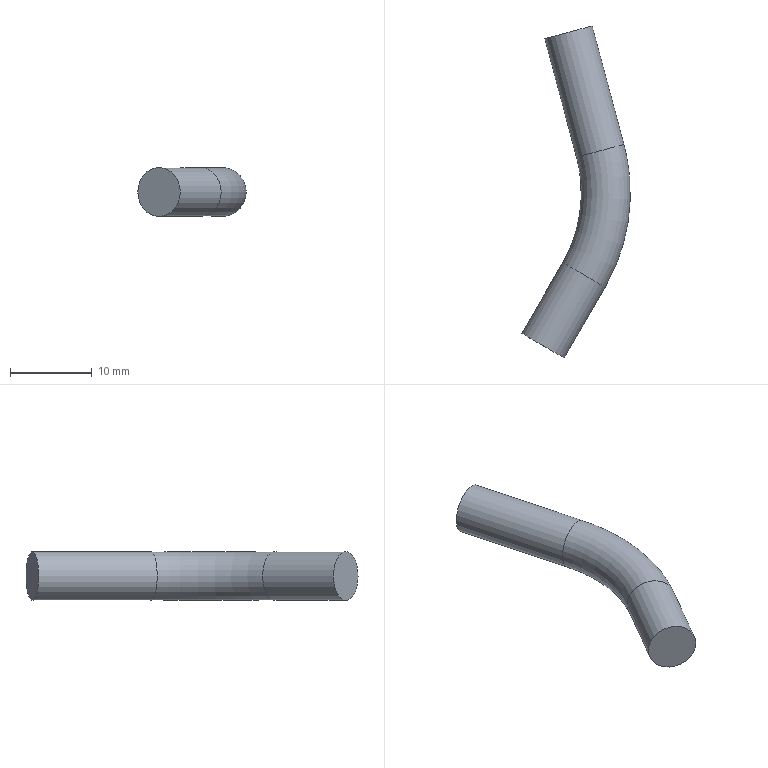Part | STEP file | 1 solid | 5 faces | box 13.278 x 40.602 x 6 mm | volume 1151 mm3 | plane 2 | cylinder 2 | torus 1 | commonest cylinder face diameters 6 x2
STEP:
#1=CARTESIAN_POINT('',(46.123,-4.113,-8.25));
#2=VERTEX_POINT('',#1);
#3=CARTESIAN_POINT('',(43.525,-2.613,-8.25));
#4=DIRECTION('',(-0.5,-0.866,0.));
#5=DIRECTION('',(0.866,-0.5,0.));
#6=AXIS2_PLACEMENT_3D('',#3,#4,#5);
#7=CIRCLE('',#6,3.);
#8=EDGE_CURVE('',#2,#2,#7,.T.);
#9=ORIENTED_EDGE('',*,*,#8,.T.);
#10=EDGE_LOOP('',(#9));
#11=FACE_BOUND('',#10,.T.);
#12=CARTESIAN_POINT('',(43.525,-2.613,-8.25));
#13=DIRECTION('',(0.5,0.866,0.));
#14=DIRECTION('',(0.,0.,-1.));
#15=AXIS2_PLACEMENT_3D('',#12,#13,#14);
#16=PLANE('',#15);
#17=ADVANCED_FACE('',(#11),#16,.F.);
#18=CARTESIAN_POINT('',(45.927,7.548,-8.25));
#19=VERTEX_POINT('',#18);
#20=CARTESIAN_POINT('',(51.123,4.548,-8.25));
#21=VERTEX_POINT('',#20);
#22=CARTESIAN_POINT('',(48.525,6.048,-8.25));
#23=DIRECTION('',(0.5,0.866,0.));
#24=DIRECTION('',(-0.866,0.5,0.));
#25=AXIS2_PLACEMENT_3D('',#22,#23,#24);
#26=CIRCLE('',#25,3.);
#27=EDGE_CURVE('',#19,#21,#26,.T.);
#28=ORIENTED_EDGE('',*,*,#27,.F.);
#29=CARTESIAN_POINT('',(48.525,6.048,-8.25));
#30=DIRECTION('',(0.5,0.866,0.));
#31=DIRECTION('',(0.866,-0.5,0.));
#32=AXIS2_PLACEMENT_3D('',#29,#30,#31);
#33=CIRCLE('',#32,3.);
#34=EDGE_CURVE('',#21,#19,#33,.T.);
#35=ORIENTED_EDGE('',*,*,#34,.F.);
#36=EDGE_LOOP('',(#28,#35));
#37=FACE_BOUND('',#36,.T.);
#38=ORIENTED_EDGE('',*,*,#8,.F.);
#39=EDGE_LOOP('',(#38));
#40=FACE_OUTER_BOUND('',#39,.T.);
#41=CARTESIAN_POINT('',(43.525,-2.613,-8.25));
#42=DIRECTION('',(-0.5,-0.866,0.));
#43=DIRECTION('',(0.866,-0.5,0.));
#44=AXIS2_PLACEMENT_3D('',#41,#42,#43);
#45=CYLINDRICAL_SURFACE('',#44,3.);
#46=ADVANCED_FACE('',(#37,#40),#45,.T.);
#47=CARTESIAN_POINT('',(53.421,22.001,-8.25));
#48=VERTEX_POINT('',#47);
#49=CARTESIAN_POINT('',(47.625,20.448,-8.25));
#50=VERTEX_POINT('',#49);
#51=CARTESIAN_POINT('',(50.523,21.224,-8.25));
#52=DIRECTION('',(0.2588,-0.9659,0.));
#53=DIRECTION('',(0.9659,0.2588,0.));
#54=AXIS2_PLACEMENT_3D('',#51,#52,#53);
#55=CIRCLE('',#54,3.);
#56=EDGE_CURVE('',#48,#50,#55,.T.);
#57=ORIENTED_EDGE('',*,*,#56,.T.);
#58=CARTESIAN_POINT('',(50.523,21.224,-8.25));
#59=DIRECTION('',(0.2588,-0.9659,0.));
#60=DIRECTION('',(-0.9659,-0.2588,0.));
#61=AXIS2_PLACEMENT_3D('',#58,#59,#60);
#62=CIRCLE('',#61,3.);
#63=EDGE_CURVE('',#50,#48,#62,.T.);
#64=ORIENTED_EDGE('',*,*,#63,.T.);
#65=EDGE_LOOP('',(#57,#64));
#66=FACE_BOUND('',#65,.T.);
#67=ORIENTED_EDGE('',*,*,#34,.T.);
#68=ORIENTED_EDGE('',*,*,#27,.T.);
#69=EDGE_LOOP('',(#67,#68));
#70=FACE_BOUND('',#69,.T.);
#71=CARTESIAN_POINT('',(31.204,16.048,-8.25));
#72=DIRECTION('',(0.,0.,1.));
#73=DIRECTION('',(-0.866,0.5,0.));
#74=AXIS2_PLACEMENT_3D('',#71,#72,#73);
#75=TOROIDAL_SURFACE('',#74,20.,3.);
#76=ADVANCED_FACE('',(#66,#70),#75,.T.);
#77=ORIENTED_EDGE('',*,*,#63,.F.);
#78=ORIENTED_EDGE('',*,*,#56,.F.);
#79=EDGE_LOOP('',(#77,#78));
#80=FACE_BOUND('',#79,.T.);
#81=CARTESIAN_POINT('',(49.538,36.489,-8.25));
#82=VERTEX_POINT('',#81);
#83=CARTESIAN_POINT('',(46.641,35.713,-8.25));
#84=DIRECTION('',(-0.2588,0.9659,0.));
#85=DIRECTION('',(-0.9659,-0.2588,0.));
#86=AXIS2_PLACEMENT_3D('',#83,#84,#85);
#87=CIRCLE('',#86,3.);
#88=EDGE_CURVE('',#82,#82,#87,.T.);
#89=ORIENTED_EDGE('',*,*,#88,.F.);
#90=EDGE_LOOP('',(#89));
#91=FACE_OUTER_BOUND('',#90,.T.);
#92=CARTESIAN_POINT('',(50.523,21.224,-8.25));
#93=DIRECTION('',(0.2588,-0.9659,0.));
#94=DIRECTION('',(0.9659,0.2588,0.));
#95=AXIS2_PLACEMENT_3D('',#92,#93,#94);
#96=CYLINDRICAL_SURFACE('',#95,3.);
#97=ADVANCED_FACE('',(#80,#91),#96,.T.);
#98=ORIENTED_EDGE('',*,*,#88,.T.);
#99=EDGE_LOOP('',(#98));
#100=FACE_BOUND('',#99,.T.);
#101=CARTESIAN_POINT('',(46.641,35.713,-8.25));
#102=DIRECTION('',(-0.2588,0.9659,0.));
#103=DIRECTION('',(0.,0.,1.));
#104=AXIS2_PLACEMENT_3D('',#101,#102,#103);
#105=PLANE('',#104);
#106=ADVANCED_FACE('',(#100),#105,.T.);
#107=CLOSED_SHELL('',(#17,#46,#76,#97,#106));
#108=MANIFOLD_SOLID_BREP('',#107);
#109=(LENGTH_UNIT()NAMED_UNIT(*)SI_UNIT(.MILLI.,.METRE.));
#110=UNCERTAINTY_MEASURE_WITH_UNIT(LENGTH_MEASURE(0.00001),#109,'','');
#111=(NAMED_UNIT(*)PLANE_ANGLE_UNIT()SI_UNIT($,.RADIAN.));
#112=(NAMED_UNIT(*)SI_UNIT($,.STERADIAN.)SOLID_ANGLE_UNIT());
#113=(GEOMETRIC_REPRESENTATION_CONTEXT(3)GLOBAL_UNCERTAINTY_ASSIGNED_CONTEXT((#110))GLOBAL_UNIT_ASSIGNED_CONTEXT((#109,#111,#112))REPRESENTATION_CONTEXT('',''));
#114=ADVANCED_BREP_SHAPE_REPRESENTATION('',(#108),#113);